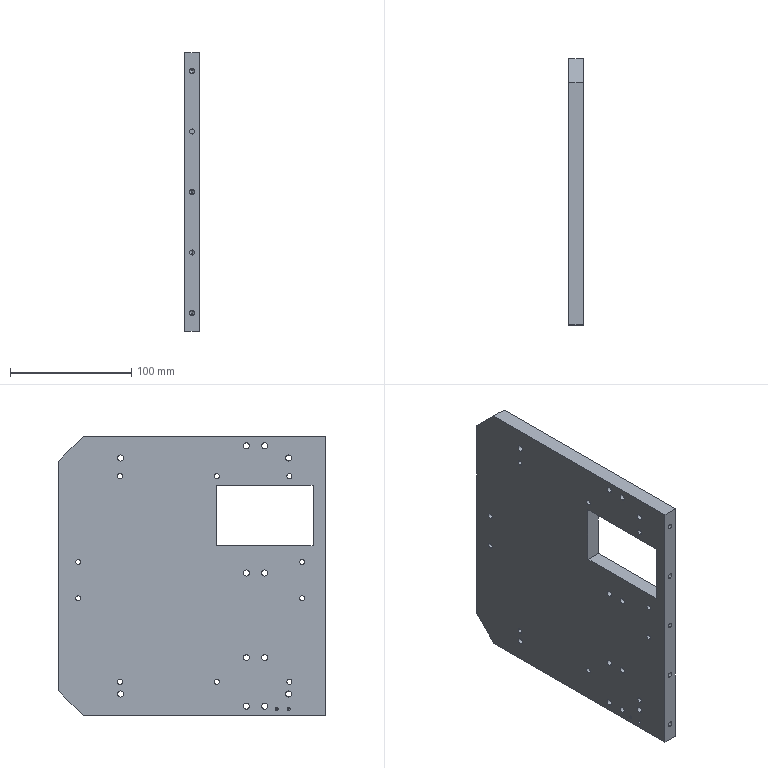Part | SolidWorks | features LPattern 12, HoleWzd 6, Chamfer 1, Extrusion 1, ICE 1 | 1 solid | 82 faces | box 12 x 220 x 230 mm | volume 548985 mm3 | cylinder 58 | cone 12 | plane 12 | commonest cylinder face diameters 4.2 x30 5 x24 2.5 x4